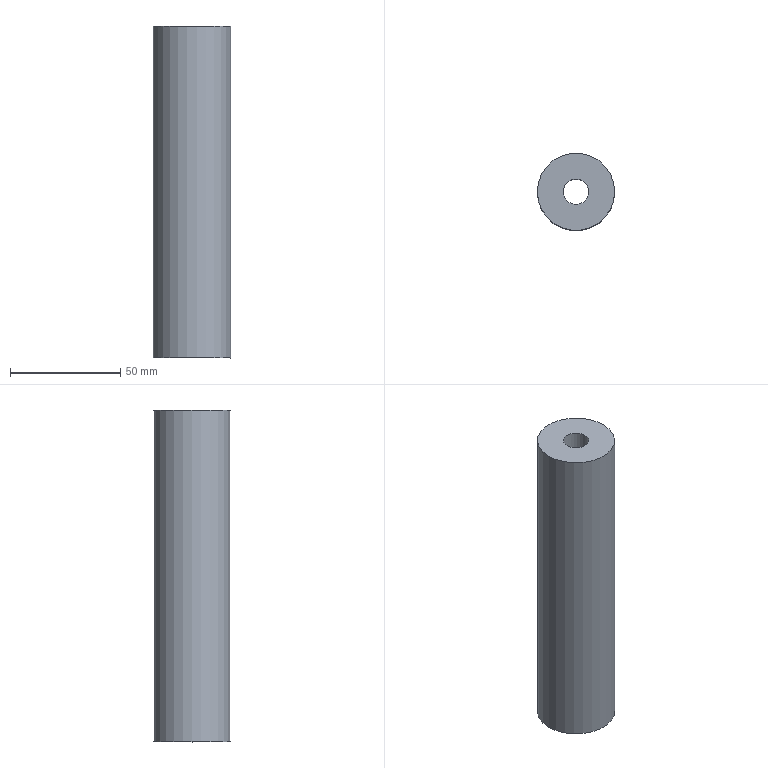Part | NX | features solid 2 | 1 solid | 6 faces | box 35 x 35 x 150.365 mm | volume 117547 mm3 | plane 3 | cylinder 3 | commonest cylinder face diameters 11.507 x1 18.008 x1 35 x1
STEP:
#1=CARTESIAN_POINT('',(885.477,189.199,64.999));
#2=VERTEX_POINT('',#1);
#3=CARTESIAN_POINT('',(867.977,189.199,64.999));
#4=DIRECTION('',(0.,0.,-1.));
#5=DIRECTION('',(1.,0.,0.));
#6=AXIS2_PLACEMENT_3D('',#3,#4,#5);
#7=CIRCLE('',#6,17.5);
#8=EDGE_CURVE('',#2,#2,#7,.F.);
#9=ORIENTED_EDGE('',*,*,#8,.T.);
#10=EDGE_LOOP('',(#9));
#11=FACE_BOUND('',#10,.T.);
#12=CARTESIAN_POINT('',(873.731,189.199,64.999));
#13=VERTEX_POINT('',#12);
#14=CARTESIAN_POINT('',(867.977,189.199,64.999));
#15=DIRECTION('',(0.,0.,-1.));
#16=DIRECTION('',(1.,0.,0.));
#17=AXIS2_PLACEMENT_3D('',#14,#15,#16);
#18=CIRCLE('',#17,5.753);
#19=EDGE_CURVE('',#13,#13,#18,.T.);
#20=ORIENTED_EDGE('',*,*,#19,.T.);
#21=EDGE_LOOP('',(#20));
#22=FACE_BOUND('',#21,.T.);
#23=CARTESIAN_POINT('',(709.977,14.199,64.999));
#24=DIRECTION('',(0.,0.,-1.));
#25=DIRECTION('',(1.,0.,0.));
#26=AXIS2_PLACEMENT_3D('',#23,#24,#25);
#27=PLANE('',#26);
#28=ADVANCED_FACE('',(#11,#22),#27,.F.);
#29=ORIENTED_EDGE('',*,*,#8,.F.);
#30=EDGE_LOOP('',(#29));
#31=FACE_BOUND('',#30,.T.);
#32=CARTESIAN_POINT('',(850.477,189.199,-85.366));
#33=VERTEX_POINT('',#32);
#34=CARTESIAN_POINT('',(867.977,189.199,-85.366));
#35=DIRECTION('',(0.,0.,-1.));
#36=DIRECTION('',(-1.,0.,0.));
#37=AXIS2_PLACEMENT_3D('',#34,#35,#36);
#38=CIRCLE('',#37,17.5);
#39=EDGE_CURVE('',#33,#33,#38,.F.);
#40=ORIENTED_EDGE('',*,*,#39,.T.);
#41=EDGE_LOOP('',(#40));
#42=FACE_BOUND('',#41,.T.);
#43=CARTESIAN_POINT('',(867.977,189.199,-26.916));
#44=DIRECTION('',(0.,0.,1.));
#45=DIRECTION('',(0.,1.,0.));
#46=AXIS2_PLACEMENT_3D('',#43,#44,#45);
#47=CYLINDRICAL_SURFACE('',#46,17.5);
#48=ADVANCED_FACE('',(#31,#42),#47,.T.);
#49=CARTESIAN_POINT('',(858.973,189.199,-85.366));
#50=VERTEX_POINT('',#49);
#51=CARTESIAN_POINT('',(867.977,189.199,-85.366));
#52=DIRECTION('',(0.,0.,-1.));
#53=DIRECTION('',(-1.,0.,0.));
#54=AXIS2_PLACEMENT_3D('',#51,#52,#53);
#55=CIRCLE('',#54,9.004);
#56=EDGE_CURVE('',#50,#50,#55,.F.);
#57=ORIENTED_EDGE('',*,*,#56,.T.);
#58=EDGE_LOOP('',(#57));
#59=FACE_BOUND('',#58,.T.);
#60=ORIENTED_EDGE('',*,*,#39,.F.);
#61=EDGE_LOOP('',(#60));
#62=FACE_BOUND('',#61,.T.);
#63=CARTESIAN_POINT('',(1131.977,165.199,-85.366));
#64=DIRECTION('',(0.,0.,-1.));
#65=DIRECTION('',(0.,1.,0.));
#66=AXIS2_PLACEMENT_3D('',#63,#64,#65);
#67=PLANE('',#66);
#68=ADVANCED_FACE('',(#59,#62),#67,.T.);
#69=CARTESIAN_POINT('',(862.224,189.199,-9.166));
#70=VERTEX_POINT('',#69);
#71=CARTESIAN_POINT('',(867.977,189.199,-9.166));
#72=DIRECTION('',(0.,0.,1.));
#73=DIRECTION('',(-1.,0.,0.));
#74=AXIS2_PLACEMENT_3D('',#71,#72,#73);
#75=CIRCLE('',#74,5.753);
#76=EDGE_CURVE('',#70,#70,#75,.T.);
#77=ORIENTED_EDGE('',*,*,#76,.F.);
#78=EDGE_LOOP('',(#77));
#79=FACE_BOUND('',#78,.T.);
#80=ORIENTED_EDGE('',*,*,#19,.F.);
#81=EDGE_LOOP('',(#80));
#82=FACE_BOUND('',#81,.T.);
#83=CARTESIAN_POINT('',(867.977,189.199,-67.166));
#84=DIRECTION('',(0.,0.,1.));
#85=DIRECTION('',(-1.,0.,0.));
#86=AXIS2_PLACEMENT_3D('',#83,#84,#85);
#87=CYLINDRICAL_SURFACE('',#86,5.753);
#88=ADVANCED_FACE('',(#79,#82),#87,.F.);
#89=ORIENTED_EDGE('',*,*,#76,.T.);
#90=EDGE_LOOP('',(#89));
#91=FACE_BOUND('',#90,.T.);
#92=CARTESIAN_POINT('',(858.973,189.199,-9.166));
#93=VERTEX_POINT('',#92);
#94=CARTESIAN_POINT('',(867.977,189.199,-9.166));
#95=DIRECTION('',(0.,0.,-1.));
#96=DIRECTION('',(-1.,0.,0.));
#97=AXIS2_PLACEMENT_3D('',#94,#95,#96);
#98=CIRCLE('',#97,9.004);
#99=EDGE_CURVE('',#93,#93,#98,.F.);
#100=ORIENTED_EDGE('',*,*,#99,.F.);
#101=EDGE_LOOP('',(#100));
#102=FACE_BOUND('',#101,.T.);
#103=CARTESIAN_POINT('',(867.977,189.199,-9.166));
#104=DIRECTION('',(0.,0.,1.));
#105=DIRECTION('',(-1.,0.,0.));
#106=AXIS2_PLACEMENT_3D('',#103,#104,#105);
#107=PLANE('',#106);
#108=ADVANCED_FACE('',(#91,#102),#107,.F.);
#109=ORIENTED_EDGE('',*,*,#99,.T.);
#110=EDGE_LOOP('',(#109));
#111=FACE_BOUND('',#110,.T.);
#112=ORIENTED_EDGE('',*,*,#56,.F.);
#113=EDGE_LOOP('',(#112));
#114=FACE_BOUND('',#113,.T.);
#115=CARTESIAN_POINT('',(867.977,189.199,-67.166));
#116=DIRECTION('',(0.,0.,1.));
#117=DIRECTION('',(-1.,0.,0.));
#118=AXIS2_PLACEMENT_3D('',#115,#116,#117);
#119=CYLINDRICAL_SURFACE('',#118,9.004);
#120=ADVANCED_FACE('',(#111,#114),#119,.F.);
#121=CLOSED_SHELL('',(#28,#48,#68,#88,#108,#120));
#122=MANIFOLD_SOLID_BREP('',#121);
#123=(LENGTH_UNIT()NAMED_UNIT(*)SI_UNIT(.MILLI.,.METRE.));
#124=UNCERTAINTY_MEASURE_WITH_UNIT(LENGTH_MEASURE(0.00001),#123,'','');
#125=(NAMED_UNIT(*)PLANE_ANGLE_UNIT()SI_UNIT($,.RADIAN.));
#126=(NAMED_UNIT(*)SI_UNIT($,.STERADIAN.)SOLID_ANGLE_UNIT());
#127=(GEOMETRIC_REPRESENTATION_CONTEXT(3)GLOBAL_UNCERTAINTY_ASSIGNED_CONTEXT((#124))GLOBAL_UNIT_ASSIGNED_CONTEXT((#123,#125,#126))REPRESENTATION_CONTEXT('',''));
#128=ADVANCED_BREP_SHAPE_REPRESENTATION('',(#122),#127);